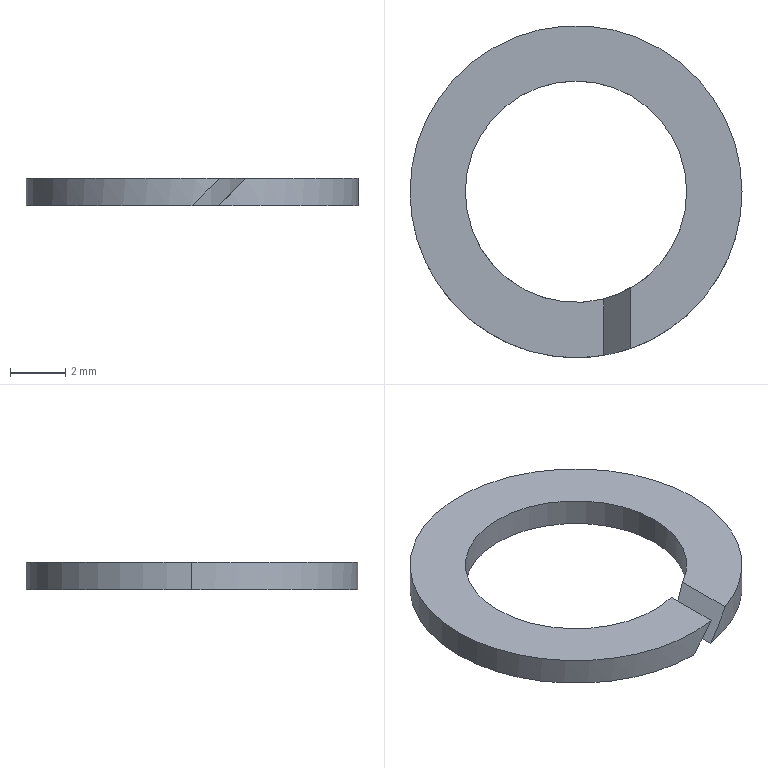Part | SolidWorks | features Extrusion 1, ICE 1 | 1 solid | 10 faces | box 12 x 12 x 1 mm | volume 60.867 mm3 | cylinder 6 | plane 4 | commonest cylinder face diameters 8 x3 12 x3
STEP:
#1=CARTESIAN_POINT('',(1.953,-3.491,1.));
#2=VERTEX_POINT('',#1);
#3=CARTESIAN_POINT('',(4.,0.,1.));
#4=VERTEX_POINT('',#3);
#5=CARTESIAN_POINT('',(0.,0.,1.));
#6=DIRECTION('',(0.,0.,1.));
#7=DIRECTION('',(1.,0.,0.));
#8=AXIS2_PLACEMENT_3D('',#5,#6,#7);
#9=CIRCLE('',#8,4.);
#10=EDGE_CURVE('',#2,#4,#9,.T.);
#11=ORIENTED_EDGE('',*,*,#10,.T.);
#12=CARTESIAN_POINT('',(4.,0.,0.));
#13=VERTEX_POINT('',#12);
#14=CARTESIAN_POINT('',(4.,0.,1.));
#15=DIRECTION('',(0.,0.,-1.));
#16=VECTOR('',#15,1000.);
#17=LINE('',#14,#16);
#18=EDGE_CURVE('',#4,#13,#17,.T.);
#19=ORIENTED_EDGE('',*,*,#18,.T.);
#20=CARTESIAN_POINT('',(0.959,-3.883,0.));
#21=VERTEX_POINT('',#20);
#22=CARTESIAN_POINT('',(0.,0.,0.));
#23=DIRECTION('',(0.,0.,1.));
#24=DIRECTION('',(1.,0.,0.));
#25=AXIS2_PLACEMENT_3D('',#22,#23,#24);
#26=CIRCLE('',#25,4.);
#27=EDGE_CURVE('',#21,#13,#26,.T.);
#28=ORIENTED_EDGE('',*,*,#27,.F.);
#29=CARTESIAN_POINT('',(1.953,-3.491,1.));
#30=CARTESIAN_POINT('',(1.64,-3.666,0.6854));
#31=CARTESIAN_POINT('',(1.307,-3.797,0.35));
#32=CARTESIAN_POINT('',(0.959,-3.883,0.));
#33=(BOUNDED_CURVE()B_SPLINE_CURVE(3,(#29,#30,#31,#32),.UNSPECIFIED.,.F.,.T.)B_SPLINE_CURVE_WITH_KNOTS((4,4),(4.202,4.47),.UNSPECIFIED.)CURVE()GEOMETRIC_REPRESENTATION_ITEM()RATIONAL_B_SPLINE_CURVE((1.,0.994,0.994,1.))REPRESENTATION_ITEM(''));
#34=EDGE_CURVE('',#2,#21,#33,.T.);
#35=ORIENTED_EDGE('',*,*,#34,.F.);
#36=EDGE_LOOP('',(#11,#19,#28,#35));
#37=FACE_OUTER_BOUND('',#36,.T.);
#38=CARTESIAN_POINT('',(0.,0.,1.));
#39=DIRECTION('',(0.,0.,-1.));
#40=DIRECTION('',(-1.,0.,0.));
#41=AXIS2_PLACEMENT_3D('',#38,#39,#40);
#42=CYLINDRICAL_SURFACE('',#41,4.);
#43=ADVANCED_FACE('',(#37),#42,.F.);
#44=ORIENTED_EDGE('',*,*,#18,.F.);
#45=CARTESIAN_POINT('',(-4.,0.,1.));
#46=VERTEX_POINT('',#45);
#47=CARTESIAN_POINT('',(0.,0.,1.));
#48=DIRECTION('',(0.,0.,1.));
#49=DIRECTION('',(1.,0.,0.));
#50=AXIS2_PLACEMENT_3D('',#47,#48,#49);
#51=CIRCLE('',#50,4.);
#52=EDGE_CURVE('',#4,#46,#51,.T.);
#53=ORIENTED_EDGE('',*,*,#52,.T.);
#54=CARTESIAN_POINT('',(-4.,0.,0.));
#55=VERTEX_POINT('',#54);
#56=CARTESIAN_POINT('',(-4.,0.,1.));
#57=DIRECTION('',(0.,0.,-1.));
#58=VECTOR('',#57,1000.);
#59=LINE('',#56,#58);
#60=EDGE_CURVE('',#46,#55,#59,.T.);
#61=ORIENTED_EDGE('',*,*,#60,.T.);
#62=CARTESIAN_POINT('',(0.,0.,0.));
#63=DIRECTION('',(0.,0.,1.));
#64=DIRECTION('',(1.,0.,0.));
#65=AXIS2_PLACEMENT_3D('',#62,#63,#64);
#66=CIRCLE('',#65,4.);
#67=EDGE_CURVE('',#13,#55,#66,.T.);
#68=ORIENTED_EDGE('',*,*,#67,.F.);
#69=EDGE_LOOP('',(#44,#53,#61,#68));
#70=FACE_OUTER_BOUND('',#69,.T.);
#71=CARTESIAN_POINT('',(0.,0.,1.));
#72=DIRECTION('',(0.,0.,-1.));
#73=DIRECTION('',(-1.,0.,0.));
#74=AXIS2_PLACEMENT_3D('',#71,#72,#73);
#75=CYLINDRICAL_SURFACE('',#74,4.);
#76=ADVANCED_FACE('',(#70),#75,.F.);
#77=CARTESIAN_POINT('',(6.,0.,1.));
#78=VERTEX_POINT('',#77);
#79=CARTESIAN_POINT('',(-6.,0.,1.));
#80=VERTEX_POINT('',#79);
#81=CARTESIAN_POINT('',(0.,0.,1.));
#82=DIRECTION('',(0.,0.,1.));
#83=DIRECTION('',(1.,0.,0.));
#84=AXIS2_PLACEMENT_3D('',#81,#82,#83);
#85=CIRCLE('',#84,6.);
#86=EDGE_CURVE('',#78,#80,#85,.T.);
#87=ORIENTED_EDGE('',*,*,#86,.F.);
#88=CARTESIAN_POINT('',(6.,0.,0.));
#89=VERTEX_POINT('',#88);
#90=CARTESIAN_POINT('',(6.,0.,1.));
#91=DIRECTION('',(0.,0.,-1.));
#92=VECTOR('',#91,1000.);
#93=LINE('',#90,#92);
#94=EDGE_CURVE('',#78,#89,#93,.T.);
#95=ORIENTED_EDGE('',*,*,#94,.T.);
#96=CARTESIAN_POINT('',(-6.,0.,0.));
#97=VERTEX_POINT('',#96);
#98=CARTESIAN_POINT('',(0.,0.,0.));
#99=DIRECTION('',(0.,0.,1.));
#100=DIRECTION('',(1.,0.,0.));
#101=AXIS2_PLACEMENT_3D('',#98,#99,#100);
#102=CIRCLE('',#101,6.);
#103=EDGE_CURVE('',#89,#97,#102,.T.);
#104=ORIENTED_EDGE('',*,*,#103,.T.);
#105=CARTESIAN_POINT('',(-6.,0.,1.));
#106=DIRECTION('',(0.,0.,-1.));
#107=VECTOR('',#106,1000.);
#108=LINE('',#105,#107);
#109=EDGE_CURVE('',#80,#97,#108,.T.);
#110=ORIENTED_EDGE('',*,*,#109,.F.);
#111=EDGE_LOOP('',(#87,#95,#104,#110));
#112=FACE_OUTER_BOUND('',#111,.T.);
#113=CARTESIAN_POINT('',(0.,0.,1.));
#114=DIRECTION('',(0.,0.,-1.));
#115=DIRECTION('',(-1.,0.,0.));
#116=AXIS2_PLACEMENT_3D('',#113,#114,#115);
#117=CYLINDRICAL_SURFACE('',#116,6.);
#118=ADVANCED_FACE('',(#112),#117,.T.);
#119=CARTESIAN_POINT('',(0.994,-5.917,1.));
#120=VERTEX_POINT('',#119);
#121=CARTESIAN_POINT('',(0.,0.,1.));
#122=DIRECTION('',(0.,0.,1.));
#123=DIRECTION('',(1.,0.,0.));
#124=AXIS2_PLACEMENT_3D('',#121,#122,#123);
#125=CIRCLE('',#124,6.);
#126=EDGE_CURVE('',#80,#120,#125,.T.);
#127=ORIENTED_EDGE('',*,*,#126,.F.);
#128=ORIENTED_EDGE('',*,*,#109,.T.);
#129=CARTESIAN_POINT('',(0.,-6.,0.));
#130=VERTEX_POINT('',#129);
#131=CARTESIAN_POINT('',(0.,0.,0.));
#132=DIRECTION('',(0.,0.,1.));
#133=DIRECTION('',(1.,0.,0.));
#134=AXIS2_PLACEMENT_3D('',#131,#132,#133);
#135=CIRCLE('',#134,6.);
#136=EDGE_CURVE('',#97,#130,#135,.T.);
#137=ORIENTED_EDGE('',*,*,#136,.T.);
#138=CARTESIAN_POINT('',(0.,-6.,0.));
#139=CARTESIAN_POINT('',(0.3333,-6.,0.3353));
#140=CARTESIAN_POINT('',(0.6654,-5.972,0.6694));
#141=CARTESIAN_POINT('',(0.994,-5.917,1.));
#142=(BOUNDED_CURVE()B_SPLINE_CURVE(3,(#138,#139,#140,#141),.UNSPECIFIED.,.F.,.T.)B_SPLINE_CURVE_WITH_KNOTS((4,4),(1.571,1.737),.UNSPECIFIED.)CURVE()GEOMETRIC_REPRESENTATION_ITEM()RATIONAL_B_SPLINE_CURVE((1.,0.9977,0.9977,1.))REPRESENTATION_ITEM(''));
#143=EDGE_CURVE('',#130,#120,#142,.T.);
#144=ORIENTED_EDGE('',*,*,#143,.T.);
#145=EDGE_LOOP('',(#127,#128,#137,#144));
#146=FACE_OUTER_BOUND('',#145,.T.);
#147=CARTESIAN_POINT('',(0.,0.,1.));
#148=DIRECTION('',(0.,0.,-1.));
#149=DIRECTION('',(-1.,0.,0.));
#150=AXIS2_PLACEMENT_3D('',#147,#148,#149);
#151=CYLINDRICAL_SURFACE('',#150,6.);
#152=ADVANCED_FACE('',(#146),#151,.T.);
#153=CARTESIAN_POINT('',(0.994,-3.875,1.));
#154=VERTEX_POINT('',#153);
#155=CARTESIAN_POINT('',(0.994,-6.,1.));
#156=DIRECTION('',(0.,1.,0.));
#157=VECTOR('',#156,1000.);
#158=LINE('',#155,#157);
#159=EDGE_CURVE('',#120,#154,#158,.T.);
#160=ORIENTED_EDGE('',*,*,#159,.T.);
#161=CARTESIAN_POINT('',(0.,0.,1.));
#162=DIRECTION('',(0.,0.,1.));
#163=DIRECTION('',(1.,0.,0.));
#164=AXIS2_PLACEMENT_3D('',#161,#162,#163);
#165=CIRCLE('',#164,4.);
#166=EDGE_CURVE('',#46,#154,#165,.T.);
#167=ORIENTED_EDGE('',*,*,#166,.F.);
#168=ORIENTED_EDGE('',*,*,#52,.F.);
#169=ORIENTED_EDGE('',*,*,#10,.F.);
#170=CARTESIAN_POINT('',(1.953,-5.673,1.));
#171=VERTEX_POINT('',#170);
#172=CARTESIAN_POINT('',(1.953,-6.,1.));
#173=DIRECTION('',(0.,1.,0.));
#174=VECTOR('',#173,1000.);
#175=LINE('',#172,#174);
#176=EDGE_CURVE('',#171,#2,#175,.T.);
#177=ORIENTED_EDGE('',*,*,#176,.F.);
#178=CARTESIAN_POINT('',(0.,0.,1.));
#179=DIRECTION('',(0.,0.,1.));
#180=DIRECTION('',(1.,0.,0.));
#181=AXIS2_PLACEMENT_3D('',#178,#179,#180);
#182=CIRCLE('',#181,6.);
#183=EDGE_CURVE('',#171,#78,#182,.T.);
#184=ORIENTED_EDGE('',*,*,#183,.T.);
#185=ORIENTED_EDGE('',*,*,#86,.T.);
#186=ORIENTED_EDGE('',*,*,#126,.T.);
#187=EDGE_LOOP('',(#160,#167,#168,#169,#177,#184,#185,#186));
#188=FACE_OUTER_BOUND('',#187,.T.);
#189=CARTESIAN_POINT('',(0.,0.,1.));
#190=DIRECTION('',(0.,0.,1.));
#191=DIRECTION('',(1.,0.,0.));
#192=AXIS2_PLACEMENT_3D('',#189,#190,#191);
#193=PLANE('',#192);
#194=ADVANCED_FACE('',(#188),#193,.T.);
#195=ORIENTED_EDGE('',*,*,#27,.T.);
#196=ORIENTED_EDGE('',*,*,#67,.T.);
#197=CARTESIAN_POINT('',(0.,-4.,0.));
#198=VERTEX_POINT('',#197);
#199=CARTESIAN_POINT('',(0.,0.,0.));
#200=DIRECTION('',(0.,0.,1.));
#201=DIRECTION('',(1.,0.,0.));
#202=AXIS2_PLACEMENT_3D('',#199,#200,#201);
#203=CIRCLE('',#202,4.);
#204=EDGE_CURVE('',#55,#198,#203,.T.);
#205=ORIENTED_EDGE('',*,*,#204,.T.);
#206=CARTESIAN_POINT('',(0.,-6.,0.));
#207=DIRECTION('',(0.,1.,0.));
#208=VECTOR('',#207,1000.);
#209=LINE('',#206,#208);
#210=EDGE_CURVE('',#130,#198,#209,.T.);
#211=ORIENTED_EDGE('',*,*,#210,.F.);
#212=ORIENTED_EDGE('',*,*,#136,.F.);
#213=ORIENTED_EDGE('',*,*,#103,.F.);
#214=CARTESIAN_POINT('',(0.959,-5.923,0.));
#215=VERTEX_POINT('',#214);
#216=CARTESIAN_POINT('',(0.,0.,0.));
#217=DIRECTION('',(0.,0.,1.));
#218=DIRECTION('',(1.,0.,0.));
#219=AXIS2_PLACEMENT_3D('',#216,#217,#218);
#220=CIRCLE('',#219,6.);
#221=EDGE_CURVE('',#215,#89,#220,.T.);
#222=ORIENTED_EDGE('',*,*,#221,.F.);
#223=CARTESIAN_POINT('',(0.959,-6.,0.));
#224=DIRECTION('',(0.,1.,0.));
#225=VECTOR('',#224,1000.);
#226=LINE('',#223,#225);
#227=EDGE_CURVE('',#215,#21,#226,.T.);
#228=ORIENTED_EDGE('',*,*,#227,.T.);
#229=EDGE_LOOP('',(#195,#196,#205,#211,#212,#213,#222,#228));
#230=FACE_OUTER_BOUND('',#229,.T.);
#231=CARTESIAN_POINT('',(0.,0.,0.));
#232=DIRECTION('',(0.,0.,1.));
#233=DIRECTION('',(1.,0.,0.));
#234=AXIS2_PLACEMENT_3D('',#231,#232,#233);
#235=PLANE('',#234);
#236=ADVANCED_FACE('',(#230),#235,.F.);
#237=ORIENTED_EDGE('',*,*,#94,.F.);
#238=ORIENTED_EDGE('',*,*,#183,.F.);
#239=CARTESIAN_POINT('',(1.953,-5.673,1.));
#240=CARTESIAN_POINT('',(1.629,-5.785,0.6742));
#241=CARTESIAN_POINT('',(1.297,-5.868,0.3401));
#242=CARTESIAN_POINT('',(0.959,-5.923,0.));
#243=(BOUNDED_CURVE()B_SPLINE_CURVE(3,(#239,#240,#241,#242),.UNSPECIFIED.,.F.,.T.)B_SPLINE_CURVE_WITH_KNOTS((4,4),(4.381,4.552),.UNSPECIFIED.)CURVE()GEOMETRIC_REPRESENTATION_ITEM()RATIONAL_B_SPLINE_CURVE((1.,0.9976,0.9976,1.))REPRESENTATION_ITEM(''));
#244=EDGE_CURVE('',#171,#215,#243,.T.);
#245=ORIENTED_EDGE('',*,*,#244,.T.);
#246=ORIENTED_EDGE('',*,*,#221,.T.);
#247=EDGE_LOOP('',(#237,#238,#245,#246));
#248=FACE_OUTER_BOUND('',#247,.T.);
#249=CARTESIAN_POINT('',(0.,0.,1.));
#250=DIRECTION('',(0.,0.,-1.));
#251=DIRECTION('',(-1.,0.,0.));
#252=AXIS2_PLACEMENT_3D('',#249,#250,#251);
#253=CYLINDRICAL_SURFACE('',#252,6.);
#254=ADVANCED_FACE('',(#248),#253,.T.);
#255=ORIENTED_EDGE('',*,*,#60,.F.);
#256=ORIENTED_EDGE('',*,*,#166,.T.);
#257=CARTESIAN_POINT('',(0.,-4.,0.));
#258=CARTESIAN_POINT('',(0.3357,-4.,0.3378));
#259=CARTESIAN_POINT('',(0.6688,-3.958,0.6728));
#260=CARTESIAN_POINT('',(0.994,-3.875,1.));
#261=(BOUNDED_CURVE()B_SPLINE_CURVE(3,(#257,#258,#259,#260),.UNSPECIFIED.,.F.,.F.)B_SPLINE_CURVE_WITH_KNOTS((4,4),(1.571,1.822),.UNSPECIFIED.)CURVE()GEOMETRIC_REPRESENTATION_ITEM()RATIONAL_B_SPLINE_CURVE((1.,0.9948,0.9948,1.))REPRESENTATION_ITEM(''));
#262=EDGE_CURVE('',#198,#154,#261,.T.);
#263=ORIENTED_EDGE('',*,*,#262,.F.);
#264=ORIENTED_EDGE('',*,*,#204,.F.);
#265=EDGE_LOOP('',(#255,#256,#263,#264));
#266=FACE_OUTER_BOUND('',#265,.T.);
#267=CARTESIAN_POINT('',(0.,0.,1.));
#268=DIRECTION('',(0.,0.,-1.));
#269=DIRECTION('',(-1.,0.,0.));
#270=AXIS2_PLACEMENT_3D('',#267,#268,#269);
#271=CYLINDRICAL_SURFACE('',#270,4.);
#272=ADVANCED_FACE('',(#266),#271,.F.);
#273=ORIENTED_EDGE('',*,*,#176,.T.);
#274=ORIENTED_EDGE('',*,*,#34,.T.);
#275=ORIENTED_EDGE('',*,*,#227,.F.);
#276=ORIENTED_EDGE('',*,*,#244,.F.);
#277=EDGE_LOOP('',(#273,#274,#275,#276));
#278=FACE_OUTER_BOUND('',#277,.T.);
#279=CARTESIAN_POINT('',(0.959,-6.,0.));
#280=DIRECTION('',(0.7092,0.,-0.705));
#281=DIRECTION('',(-0.705,0.,-0.7092));
#282=AXIS2_PLACEMENT_3D('',#279,#280,#281);
#283=PLANE('',#282);
#284=ADVANCED_FACE('',(#278),#283,.F.);
#285=ORIENTED_EDGE('',*,*,#210,.T.);
#286=ORIENTED_EDGE('',*,*,#262,.T.);
#287=ORIENTED_EDGE('',*,*,#159,.F.);
#288=ORIENTED_EDGE('',*,*,#143,.F.);
#289=EDGE_LOOP('',(#285,#286,#287,#288));
#290=FACE_OUTER_BOUND('',#289,.T.);
#291=CARTESIAN_POINT('',(0.994,-6.,1.));
#292=DIRECTION('',(-0.7092,0.,0.705));
#293=DIRECTION('',(0.705,0.,0.7092));
#294=AXIS2_PLACEMENT_3D('',#291,#292,#293);
#295=PLANE('',#294);
#296=ADVANCED_FACE('',(#290),#295,.F.);
#297=CLOSED_SHELL('',(#43,#76,#118,#152,#194,#236,#254,#272,#284,#296));
#298=MANIFOLD_SOLID_BREP('',#297);
#299=CARTESIAN_POINT('',(0.,0.,0.));
#300=DIRECTION('',(0.,0.,1.));
#301=DIRECTION('',(1.,0.,0.));
#302=AXIS2_PLACEMENT_3D('',#299,#300,#301);
#303=(LENGTH_UNIT()NAMED_UNIT(*)SI_UNIT(.MILLI.,.METRE.));
#304=UNCERTAINTY_MEASURE_WITH_UNIT(LENGTH_MEASURE(0.00001),#303,'','');
#305=(NAMED_UNIT(*)PLANE_ANGLE_UNIT()SI_UNIT($,.RADIAN.));
#306=(NAMED_UNIT(*)SI_UNIT($,.STERADIAN.)SOLID_ANGLE_UNIT());
#307=(GEOMETRIC_REPRESENTATION_CONTEXT(3)GLOBAL_UNCERTAINTY_ASSIGNED_CONTEXT((#304))GLOBAL_UNIT_ASSIGNED_CONTEXT((#303,#305,#306))REPRESENTATION_CONTEXT('',''));
#308=ADVANCED_BREP_SHAPE_REPRESENTATION('',(#298,#302),#307);